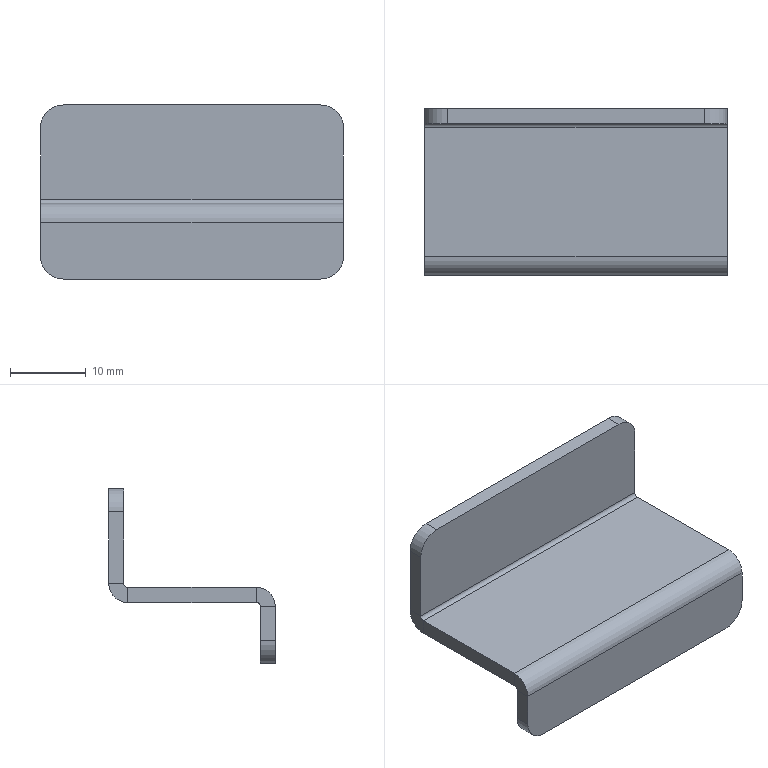Part | SolidWorks | features BaseBody 1 | 1 solid | 26 faces | box 40 x 22 x 23 mm | volume 3322 mm3 | plane 18 | cylinder 8 | commonest cylinder face diameters 6 x4 1 x2 5 x2
STEP:
#1=CARTESIAN_POINT('',(17.,-11.,-10.));
#2=VERTEX_POINT('',#1);
#3=CARTESIAN_POINT('',(20.,-11.,-7.));
#4=VERTEX_POINT('',#3);
#5=CARTESIAN_POINT('',(17.,-11.,-7.));
#6=DIRECTION('',(0.,-1.,0.));
#7=DIRECTION('',(0.,0.,-1.));
#8=AXIS2_PLACEMENT_3D('',#5,#6,#7);
#9=CIRCLE('',#8,3.);
#10=EDGE_CURVE('',#2,#4,#9,.T.);
#11=ORIENTED_EDGE('',*,*,#10,.F.);
#12=CARTESIAN_POINT('',(17.,-9.,-10.));
#13=VERTEX_POINT('',#12);
#14=CARTESIAN_POINT('',(17.,-11.,-10.));
#15=DIRECTION('',(0.,-1.,0.));
#16=VECTOR('',#15,1000.);
#17=LINE('',#14,#16);
#18=EDGE_CURVE('',#13,#2,#17,.T.);
#19=ORIENTED_EDGE('',*,*,#18,.F.);
#20=CARTESIAN_POINT('',(20.,-9.,-7.));
#21=VERTEX_POINT('',#20);
#22=CARTESIAN_POINT('',(17.,-9.,-7.));
#23=DIRECTION('',(0.,1.,0.));
#24=DIRECTION('',(0.,0.,-1.));
#25=AXIS2_PLACEMENT_3D('',#22,#23,#24);
#26=CIRCLE('',#25,3.);
#27=EDGE_CURVE('',#21,#13,#26,.T.);
#28=ORIENTED_EDGE('',*,*,#27,.F.);
#29=CARTESIAN_POINT('',(20.,-11.,-7.));
#30=DIRECTION('',(0.,1.,0.));
#31=VECTOR('',#30,1000.);
#32=LINE('',#29,#31);
#33=EDGE_CURVE('',#4,#21,#32,.T.);
#34=ORIENTED_EDGE('',*,*,#33,.F.);
#35=EDGE_LOOP('',(#11,#19,#28,#34));
#36=FACE_OUTER_BOUND('',#35,.T.);
#37=CARTESIAN_POINT('',(17.,-11.,-7.));
#38=DIRECTION('',(0.,1.,0.));
#39=DIRECTION('',(0.,0.,1.));
#40=AXIS2_PLACEMENT_3D('',#37,#38,#39);
#41=CYLINDRICAL_SURFACE('',#40,3.);
#42=ADVANCED_FACE('',(#36),#41,.T.);
#43=CARTESIAN_POINT('',(-20.,-11.,-7.));
#44=VERTEX_POINT('',#43);
#45=CARTESIAN_POINT('',(-17.,-11.,-10.));
#46=VERTEX_POINT('',#45);
#47=CARTESIAN_POINT('',(-17.,-11.,-7.));
#48=DIRECTION('',(0.,-1.,0.));
#49=DIRECTION('',(0.,0.,-1.));
#50=AXIS2_PLACEMENT_3D('',#47,#48,#49);
#51=CIRCLE('',#50,3.);
#52=EDGE_CURVE('',#44,#46,#51,.T.);
#53=ORIENTED_EDGE('',*,*,#52,.F.);
#54=CARTESIAN_POINT('',(-20.,-9.,-7.));
#55=VERTEX_POINT('',#54);
#56=CARTESIAN_POINT('',(-20.,-11.,-7.));
#57=DIRECTION('',(0.,-1.,0.));
#58=VECTOR('',#57,1000.);
#59=LINE('',#56,#58);
#60=EDGE_CURVE('',#55,#44,#59,.T.);
#61=ORIENTED_EDGE('',*,*,#60,.F.);
#62=CARTESIAN_POINT('',(-17.,-9.,-10.));
#63=VERTEX_POINT('',#62);
#64=CARTESIAN_POINT('',(-17.,-9.,-7.));
#65=DIRECTION('',(0.,1.,0.));
#66=DIRECTION('',(0.,0.,-1.));
#67=AXIS2_PLACEMENT_3D('',#64,#65,#66);
#68=CIRCLE('',#67,3.);
#69=EDGE_CURVE('',#63,#55,#68,.T.);
#70=ORIENTED_EDGE('',*,*,#69,.F.);
#71=CARTESIAN_POINT('',(-17.,-11.,-10.));
#72=DIRECTION('',(0.,1.,0.));
#73=VECTOR('',#72,1000.);
#74=LINE('',#71,#73);
#75=EDGE_CURVE('',#46,#63,#74,.T.);
#76=ORIENTED_EDGE('',*,*,#75,.F.);
#77=EDGE_LOOP('',(#53,#61,#70,#76));
#78=FACE_OUTER_BOUND('',#77,.T.);
#79=CARTESIAN_POINT('',(-17.,-11.,-7.));
#80=DIRECTION('',(0.,1.,0.));
#81=DIRECTION('',(0.,0.,1.));
#82=AXIS2_PLACEMENT_3D('',#79,#80,#81);
#83=CYLINDRICAL_SURFACE('',#82,3.);
#84=ADVANCED_FACE('',(#78),#83,.T.);
#85=CARTESIAN_POINT('',(17.,11.,13.));
#86=VERTEX_POINT('',#85);
#87=CARTESIAN_POINT('',(20.,11.,10.));
#88=VERTEX_POINT('',#87);
#89=CARTESIAN_POINT('',(17.,11.,10.));
#90=DIRECTION('',(0.,1.,0.));
#91=DIRECTION('',(0.,0.,-1.));
#92=AXIS2_PLACEMENT_3D('',#89,#90,#91);
#93=CIRCLE('',#92,3.);
#94=EDGE_CURVE('',#86,#88,#93,.T.);
#95=ORIENTED_EDGE('',*,*,#94,.F.);
#96=CARTESIAN_POINT('',(17.,9.,13.));
#97=VERTEX_POINT('',#96);
#98=CARTESIAN_POINT('',(17.,11.,13.));
#99=DIRECTION('',(0.,1.,0.));
#100=VECTOR('',#99,1000.);
#101=LINE('',#98,#100);
#102=EDGE_CURVE('',#97,#86,#101,.T.);
#103=ORIENTED_EDGE('',*,*,#102,.F.);
#104=CARTESIAN_POINT('',(20.,9.,10.));
#105=VERTEX_POINT('',#104);
#106=CARTESIAN_POINT('',(17.,9.,10.));
#107=DIRECTION('',(0.,-1.,0.));
#108=DIRECTION('',(0.,0.,-1.));
#109=AXIS2_PLACEMENT_3D('',#106,#107,#108);
#110=CIRCLE('',#109,3.);
#111=EDGE_CURVE('',#105,#97,#110,.T.);
#112=ORIENTED_EDGE('',*,*,#111,.F.);
#113=CARTESIAN_POINT('',(20.,11.,10.));
#114=DIRECTION('',(0.,-1.,0.));
#115=VECTOR('',#114,1000.);
#116=LINE('',#113,#115);
#117=EDGE_CURVE('',#88,#105,#116,.T.);
#118=ORIENTED_EDGE('',*,*,#117,.F.);
#119=EDGE_LOOP('',(#95,#103,#112,#118));
#120=FACE_OUTER_BOUND('',#119,.T.);
#121=CARTESIAN_POINT('',(17.,11.,10.));
#122=DIRECTION('',(0.,-1.,0.));
#123=DIRECTION('',(0.,0.,-1.));
#124=AXIS2_PLACEMENT_3D('',#121,#122,#123);
#125=CYLINDRICAL_SURFACE('',#124,3.);
#126=ADVANCED_FACE('',(#120),#125,.T.);
#127=CARTESIAN_POINT('',(-20.,11.,10.));
#128=VERTEX_POINT('',#127);
#129=CARTESIAN_POINT('',(-17.,11.,13.));
#130=VERTEX_POINT('',#129);
#131=CARTESIAN_POINT('',(-17.,11.,10.));
#132=DIRECTION('',(0.,1.,0.));
#133=DIRECTION('',(0.,0.,-1.));
#134=AXIS2_PLACEMENT_3D('',#131,#132,#133);
#135=CIRCLE('',#134,3.);
#136=EDGE_CURVE('',#128,#130,#135,.T.);
#137=ORIENTED_EDGE('',*,*,#136,.F.);
#138=CARTESIAN_POINT('',(-20.,9.,10.));
#139=VERTEX_POINT('',#138);
#140=CARTESIAN_POINT('',(-20.,11.,10.));
#141=DIRECTION('',(0.,1.,0.));
#142=VECTOR('',#141,1000.);
#143=LINE('',#140,#142);
#144=EDGE_CURVE('',#139,#128,#143,.T.);
#145=ORIENTED_EDGE('',*,*,#144,.F.);
#146=CARTESIAN_POINT('',(-17.,9.,13.));
#147=VERTEX_POINT('',#146);
#148=CARTESIAN_POINT('',(-17.,9.,10.));
#149=DIRECTION('',(0.,-1.,0.));
#150=DIRECTION('',(0.,0.,-1.));
#151=AXIS2_PLACEMENT_3D('',#148,#149,#150);
#152=CIRCLE('',#151,3.);
#153=EDGE_CURVE('',#147,#139,#152,.T.);
#154=ORIENTED_EDGE('',*,*,#153,.F.);
#155=CARTESIAN_POINT('',(-17.,11.,13.));
#156=DIRECTION('',(0.,-1.,0.));
#157=VECTOR('',#156,1000.);
#158=LINE('',#155,#157);
#159=EDGE_CURVE('',#130,#147,#158,.T.);
#160=ORIENTED_EDGE('',*,*,#159,.F.);
#161=EDGE_LOOP('',(#137,#145,#154,#160));
#162=FACE_OUTER_BOUND('',#161,.T.);
#163=CARTESIAN_POINT('',(-17.,11.,10.));
#164=DIRECTION('',(0.,-1.,0.));
#165=DIRECTION('',(0.,0.,-1.));
#166=AXIS2_PLACEMENT_3D('',#163,#164,#165);
#167=CYLINDRICAL_SURFACE('',#166,3.);
#168=ADVANCED_FACE('',(#162),#167,.T.);
#169=CARTESIAN_POINT('',(0.,11.,13.));
#170=DIRECTION('',(1.,0.,0.));
#171=VECTOR('',#170,1000.);
#172=LINE('',#169,#171);
#173=EDGE_CURVE('',#130,#86,#172,.T.);
#174=ORIENTED_EDGE('',*,*,#173,.F.);
#175=ORIENTED_EDGE('',*,*,#159,.T.);
#176=CARTESIAN_POINT('',(20.,9.,13.));
#177=DIRECTION('',(1.,0.,0.));
#178=VECTOR('',#177,1000.);
#179=LINE('',#176,#178);
#180=EDGE_CURVE('',#147,#97,#179,.T.);
#181=ORIENTED_EDGE('',*,*,#180,.T.);
#182=ORIENTED_EDGE('',*,*,#102,.T.);
#183=EDGE_LOOP('',(#174,#175,#181,#182));
#184=FACE_OUTER_BOUND('',#183,.T.);
#185=CARTESIAN_POINT('',(20.,11.,13.));
#186=DIRECTION('',(0.,0.,-1.));
#187=DIRECTION('',(0.,-1.,0.));
#188=AXIS2_PLACEMENT_3D('',#185,#186,#187);
#189=PLANE('',#188);
#190=ADVANCED_FACE('',(#184),#189,.F.);
#191=ORIENTED_EDGE('',*,*,#180,.F.);
#192=ORIENTED_EDGE('',*,*,#153,.T.);
#193=CARTESIAN_POINT('',(-20.,9.,0.5));
#194=VERTEX_POINT('',#193);
#195=CARTESIAN_POINT('',(-20.,9.,13.));
#196=DIRECTION('',(0.,0.,1.));
#197=VECTOR('',#196,1000.);
#198=LINE('',#195,#197);
#199=EDGE_CURVE('',#194,#139,#198,.T.);
#200=ORIENTED_EDGE('',*,*,#199,.F.);
#201=CARTESIAN_POINT('',(20.,9.,0.5));
#202=VERTEX_POINT('',#201);
#203=CARTESIAN_POINT('',(20.,9.,0.5));
#204=DIRECTION('',(-1.,0.,0.));
#205=VECTOR('',#204,1000.);
#206=LINE('',#203,#205);
#207=EDGE_CURVE('',#202,#194,#206,.T.);
#208=ORIENTED_EDGE('',*,*,#207,.F.);
#209=CARTESIAN_POINT('',(20.,9.,0.));
#210=DIRECTION('',(0.,0.,-1.));
#211=VECTOR('',#210,1000.);
#212=LINE('',#209,#211);
#213=EDGE_CURVE('',#105,#202,#212,.T.);
#214=ORIENTED_EDGE('',*,*,#213,.F.);
#215=ORIENTED_EDGE('',*,*,#111,.T.);
#216=EDGE_LOOP('',(#191,#192,#200,#208,#214,#215));
#217=FACE_OUTER_BOUND('',#216,.T.);
#218=CARTESIAN_POINT('',(0.,9.,0.));
#219=DIRECTION('',(0.,-1.,0.));
#220=DIRECTION('',(-1.,0.,0.));
#221=AXIS2_PLACEMENT_3D('',#218,#219,#220);
#222=PLANE('',#221);
#223=ADVANCED_FACE('',(#217),#222,.T.);
#224=CARTESIAN_POINT('',(-20.,11.,0.5));
#225=VERTEX_POINT('',#224);
#226=CARTESIAN_POINT('',(-20.,11.,0.));
#227=DIRECTION('',(0.,0.,1.));
#228=VECTOR('',#227,1000.);
#229=LINE('',#226,#228);
#230=EDGE_CURVE('',#225,#128,#229,.T.);
#231=ORIENTED_EDGE('',*,*,#230,.T.);
#232=ORIENTED_EDGE('',*,*,#136,.T.);
#233=ORIENTED_EDGE('',*,*,#173,.T.);
#234=ORIENTED_EDGE('',*,*,#94,.T.);
#235=CARTESIAN_POINT('',(20.,11.,0.5));
#236=VERTEX_POINT('',#235);
#237=CARTESIAN_POINT('',(20.,11.,0.));
#238=DIRECTION('',(0.,0.,-1.));
#239=VECTOR('',#238,1000.);
#240=LINE('',#237,#239);
#241=EDGE_CURVE('',#88,#236,#240,.T.);
#242=ORIENTED_EDGE('',*,*,#241,.T.);
#243=CARTESIAN_POINT('',(20.,11.,0.5));
#244=DIRECTION('',(1.,0.,0.));
#245=VECTOR('',#244,1000.);
#246=LINE('',#243,#245);
#247=EDGE_CURVE('',#225,#236,#246,.T.);
#248=ORIENTED_EDGE('',*,*,#247,.F.);
#249=EDGE_LOOP('',(#231,#232,#233,#234,#242,#248));
#250=FACE_OUTER_BOUND('',#249,.T.);
#251=CARTESIAN_POINT('',(0.,11.,0.));
#252=DIRECTION('',(0.,-1.,0.));
#253=DIRECTION('',(-1.,0.,0.));
#254=AXIS2_PLACEMENT_3D('',#251,#252,#253);
#255=PLANE('',#254);
#256=ADVANCED_FACE('',(#250),#255,.F.);
#257=ORIENTED_EDGE('',*,*,#199,.T.);
#258=ORIENTED_EDGE('',*,*,#144,.T.);
#259=ORIENTED_EDGE('',*,*,#230,.F.);
#260=CARTESIAN_POINT('',(-20.,9.,0.5));
#261=DIRECTION('',(0.,1.,0.));
#262=VECTOR('',#261,1000.);
#263=LINE('',#260,#262);
#264=EDGE_CURVE('',#194,#225,#263,.T.);
#265=ORIENTED_EDGE('',*,*,#264,.F.);
#266=EDGE_LOOP('',(#257,#258,#259,#265));
#267=FACE_OUTER_BOUND('',#266,.T.);
#268=CARTESIAN_POINT('',(-20.,11.,13.));
#269=DIRECTION('',(1.,0.,0.));
#270=DIRECTION('',(0.,1.,0.));
#271=AXIS2_PLACEMENT_3D('',#268,#269,#270);
#272=PLANE('',#271);
#273=ADVANCED_FACE('',(#267),#272,.F.);
#274=ORIENTED_EDGE('',*,*,#241,.F.);
#275=ORIENTED_EDGE('',*,*,#117,.T.);
#276=ORIENTED_EDGE('',*,*,#213,.T.);
#277=CARTESIAN_POINT('',(20.,11.,0.5));
#278=DIRECTION('',(0.,1.,0.));
#279=VECTOR('',#278,1000.);
#280=LINE('',#277,#279);
#281=EDGE_CURVE('',#202,#236,#280,.T.);
#282=ORIENTED_EDGE('',*,*,#281,.T.);
#283=EDGE_LOOP('',(#274,#275,#276,#282));
#284=FACE_OUTER_BOUND('',#283,.T.);
#285=CARTESIAN_POINT('',(20.,11.,0.));
#286=DIRECTION('',(-1.,0.,0.));
#287=DIRECTION('',(0.,0.,1.));
#288=AXIS2_PLACEMENT_3D('',#285,#286,#287);
#289=PLANE('',#288);
#290=ADVANCED_FACE('',(#284),#289,.F.);
#291=CARTESIAN_POINT('',(-20.,8.5,0.));
#292=VERTEX_POINT('',#291);
#293=CARTESIAN_POINT('',(20.,8.5,0.));
#294=VERTEX_POINT('',#293);
#295=CARTESIAN_POINT('',(-20.,8.5,0.));
#296=DIRECTION('',(1.,0.,0.));
#297=VECTOR('',#296,1000.);
#298=LINE('',#295,#297);
#299=EDGE_CURVE('',#292,#294,#298,.T.);
#300=ORIENTED_EDGE('',*,*,#299,.T.);
#301=CARTESIAN_POINT('',(20.,8.5,0.5));
#302=DIRECTION('',(1.,0.,0.));
#303=DIRECTION('',(0.,0.,1.));
#304=AXIS2_PLACEMENT_3D('',#301,#302,#303);
#305=CIRCLE('',#304,0.5);
#306=EDGE_CURVE('',#294,#202,#305,.T.);
#307=ORIENTED_EDGE('',*,*,#306,.T.);
#308=ORIENTED_EDGE('',*,*,#207,.T.);
#309=CARTESIAN_POINT('',(-20.,8.5,0.5));
#310=DIRECTION('',(-1.,0.,0.));
#311=DIRECTION('',(0.,0.,1.));
#312=AXIS2_PLACEMENT_3D('',#309,#310,#311);
#313=CIRCLE('',#312,0.5);
#314=EDGE_CURVE('',#194,#292,#313,.T.);
#315=ORIENTED_EDGE('',*,*,#314,.T.);
#316=EDGE_LOOP('',(#300,#307,#308,#315));
#317=FACE_OUTER_BOUND('',#316,.T.);
#318=CARTESIAN_POINT('',(-20.,8.5,0.5));
#319=DIRECTION('',(-1.,0.,0.));
#320=DIRECTION('',(0.,1.,0.));
#321=AXIS2_PLACEMENT_3D('',#318,#319,#320);
#322=CYLINDRICAL_SURFACE('',#321,0.5);
#323=ADVANCED_FACE('',(#317),#322,.F.);
#324=CARTESIAN_POINT('',(-20.,8.5,-2.));
#325=VERTEX_POINT('',#324);
#326=CARTESIAN_POINT('',(20.,8.5,-2.));
#327=VERTEX_POINT('',#326);
#328=CARTESIAN_POINT('',(-20.,8.5,-2.));
#329=DIRECTION('',(1.,0.,0.));
#330=VECTOR('',#329,1000.);
#331=LINE('',#328,#330);
#332=EDGE_CURVE('',#325,#327,#331,.T.);
#333=ORIENTED_EDGE('',*,*,#332,.F.);
#334=CARTESIAN_POINT('',(-20.,8.5,0.5));
#335=DIRECTION('',(-1.,0.,0.));
#336=DIRECTION('',(0.,0.,1.));
#337=AXIS2_PLACEMENT_3D('',#334,#335,#336);
#338=CIRCLE('',#337,2.5);
#339=EDGE_CURVE('',#225,#325,#338,.T.);
#340=ORIENTED_EDGE('',*,*,#339,.F.);
#341=ORIENTED_EDGE('',*,*,#247,.T.);
#342=CARTESIAN_POINT('',(20.,8.5,0.5));
#343=DIRECTION('',(1.,0.,0.));
#344=DIRECTION('',(0.,0.,1.));
#345=AXIS2_PLACEMENT_3D('',#342,#343,#344);
#346=CIRCLE('',#345,2.5);
#347=EDGE_CURVE('',#327,#236,#346,.T.);
#348=ORIENTED_EDGE('',*,*,#347,.F.);
#349=EDGE_LOOP('',(#333,#340,#341,#348));
#350=FACE_OUTER_BOUND('',#349,.T.);
#351=CARTESIAN_POINT('',(-20.,8.5,0.5));
#352=DIRECTION('',(-1.,0.,0.));
#353=DIRECTION('',(0.,1.,0.));
#354=AXIS2_PLACEMENT_3D('',#351,#352,#353);
#355=CYLINDRICAL_SURFACE('',#354,2.5);
#356=ADVANCED_FACE('',(#350),#355,.T.);
#357=ORIENTED_EDGE('',*,*,#314,.F.);
#358=ORIENTED_EDGE('',*,*,#264,.T.);
#359=ORIENTED_EDGE('',*,*,#339,.T.);
#360=CARTESIAN_POINT('',(-20.,8.5,0.));
#361=DIRECTION('',(0.,0.,-1.));
#362=VECTOR('',#361,1000.);
#363=LINE('',#360,#362);
#364=EDGE_CURVE('',#292,#325,#363,.T.);
#365=ORIENTED_EDGE('',*,*,#364,.F.);
#366=EDGE_LOOP('',(#357,#358,#359,#365));
#367=FACE_OUTER_BOUND('',#366,.T.);
#368=CARTESIAN_POINT('',(-20.,8.5,0.5));
#369=DIRECTION('',(1.,0.,0.));
#370=DIRECTION('',(0.,1.,0.));
#371=AXIS2_PLACEMENT_3D('',#368,#369,#370);
#372=PLANE('',#371);
#373=ADVANCED_FACE('',(#367),#372,.F.);
#374=ORIENTED_EDGE('',*,*,#281,.F.);
#375=ORIENTED_EDGE('',*,*,#306,.F.);
#376=CARTESIAN_POINT('',(20.,8.5,0.));
#377=DIRECTION('',(0.,0.,-1.));
#378=VECTOR('',#377,1000.);
#379=LINE('',#376,#378);
#380=EDGE_CURVE('',#294,#327,#379,.T.);
#381=ORIENTED_EDGE('',*,*,#380,.T.);
#382=ORIENTED_EDGE('',*,*,#347,.T.);
#383=EDGE_LOOP('',(#374,#375,#381,#382));
#384=FACE_OUTER_BOUND('',#383,.T.);
#385=CARTESIAN_POINT('',(20.,8.5,0.5));
#386=DIRECTION('',(1.,0.,0.));
#387=DIRECTION('',(0.,1.,0.));
#388=AXIS2_PLACEMENT_3D('',#385,#386,#387);
#389=PLANE('',#388);
#390=ADVANCED_FACE('',(#384),#389,.T.);
#391=CARTESIAN_POINT('',(-20.,-11.,-10.));
#392=DIRECTION('',(-1.,0.,0.));
#393=VECTOR('',#392,1000.);
#394=LINE('',#391,#393);
#395=EDGE_CURVE('',#2,#46,#394,.T.);
#396=ORIENTED_EDGE('',*,*,#395,.T.);
#397=ORIENTED_EDGE('',*,*,#75,.T.);
#398=CARTESIAN_POINT('',(0.,-9.,-10.));
#399=DIRECTION('',(-1.,0.,0.));
#400=VECTOR('',#399,1000.);
#401=LINE('',#398,#400);
#402=EDGE_CURVE('',#13,#63,#401,.T.);
#403=ORIENTED_EDGE('',*,*,#402,.F.);
#404=ORIENTED_EDGE('',*,*,#18,.T.);
#405=EDGE_LOOP('',(#396,#397,#403,#404));
#406=FACE_OUTER_BOUND('',#405,.T.);
#407=CARTESIAN_POINT('',(-20.,-11.,-10.));
#408=DIRECTION('',(0.,0.,-1.));
#409=DIRECTION('',(0.,-1.,0.));
#410=AXIS2_PLACEMENT_3D('',#407,#408,#409);
#411=PLANE('',#410);
#412=ADVANCED_FACE('',(#406),#411,.T.);
#413=ORIENTED_EDGE('',*,*,#402,.T.);
#414=ORIENTED_EDGE('',*,*,#69,.T.);
#415=CARTESIAN_POINT('',(-20.,-9.,-2.5));
#416=VERTEX_POINT('',#415);
#417=CARTESIAN_POINT('',(-20.,-9.,0.));
#418=DIRECTION('',(0.,0.,1.));
#419=VECTOR('',#418,1000.);
#420=LINE('',#417,#419);
#421=EDGE_CURVE('',#55,#416,#420,.T.);
#422=ORIENTED_EDGE('',*,*,#421,.T.);
#423=CARTESIAN_POINT('',(20.,-9.,-2.5));
#424=VERTEX_POINT('',#423);
#425=CARTESIAN_POINT('',(20.,-9.,-2.5));
#426=DIRECTION('',(-1.,0.,0.));
#427=VECTOR('',#426,1000.);
#428=LINE('',#425,#427);
#429=EDGE_CURVE('',#424,#416,#428,.T.);
#430=ORIENTED_EDGE('',*,*,#429,.F.);
#431=CARTESIAN_POINT('',(20.,-9.,0.));
#432=DIRECTION('',(0.,0.,-1.));
#433=VECTOR('',#432,1000.);
#434=LINE('',#431,#433);
#435=EDGE_CURVE('',#424,#21,#434,.T.);
#436=ORIENTED_EDGE('',*,*,#435,.T.);
#437=ORIENTED_EDGE('',*,*,#27,.T.);
#438=EDGE_LOOP('',(#413,#414,#422,#430,#436,#437));
#439=FACE_OUTER_BOUND('',#438,.T.);
#440=CARTESIAN_POINT('',(0.,-9.,0.));
#441=DIRECTION('',(0.,-1.,0.));
#442=DIRECTION('',(-1.,0.,0.));
#443=AXIS2_PLACEMENT_3D('',#440,#441,#442);
#444=PLANE('',#443);
#445=ADVANCED_FACE('',(#439),#444,.F.);
#446=CARTESIAN_POINT('',(-20.,-11.,-2.5));
#447=VERTEX_POINT('',#446);
#448=CARTESIAN_POINT('',(-20.,-11.,-2.));
#449=DIRECTION('',(0.,0.,1.));
#450=VECTOR('',#449,1000.);
#451=LINE('',#448,#450);
#452=EDGE_CURVE('',#44,#447,#451,.T.);
#453=ORIENTED_EDGE('',*,*,#452,.F.);
#454=ORIENTED_EDGE('',*,*,#52,.T.);
#455=ORIENTED_EDGE('',*,*,#395,.F.);
#456=ORIENTED_EDGE('',*,*,#10,.T.);
#457=CARTESIAN_POINT('',(20.,-11.,-2.5));
#458=VERTEX_POINT('',#457);
#459=CARTESIAN_POINT('',(20.,-11.,-10.));
#460=DIRECTION('',(0.,0.,-1.));
#461=VECTOR('',#460,1000.);
#462=LINE('',#459,#461);
#463=EDGE_CURVE('',#458,#4,#462,.T.);
#464=ORIENTED_EDGE('',*,*,#463,.F.);
#465=CARTESIAN_POINT('',(0.,-11.,-2.5));
#466=DIRECTION('',(-1.,0.,0.));
#467=VECTOR('',#466,1000.);
#468=LINE('',#465,#467);
#469=EDGE_CURVE('',#458,#447,#468,.T.);
#470=ORIENTED_EDGE('',*,*,#469,.T.);
#471=EDGE_LOOP('',(#453,#454,#455,#456,#464,#470));
#472=FACE_OUTER_BOUND('',#471,.T.);
#473=CARTESIAN_POINT('',(0.,-11.,0.));
#474=DIRECTION('',(0.,-1.,0.));
#475=DIRECTION('',(-1.,0.,0.));
#476=AXIS2_PLACEMENT_3D('',#473,#474,#475);
#477=PLANE('',#476);
#478=ADVANCED_FACE('',(#472),#477,.T.);
#479=ORIENTED_EDGE('',*,*,#463,.T.);
#480=ORIENTED_EDGE('',*,*,#33,.T.);
#481=ORIENTED_EDGE('',*,*,#435,.F.);
#482=CARTESIAN_POINT('',(20.,-11.,-2.5));
#483=DIRECTION('',(0.,-1.,0.));
#484=VECTOR('',#483,1000.);
#485=LINE('',#482,#484);
#486=EDGE_CURVE('',#424,#458,#485,.T.);
#487=ORIENTED_EDGE('',*,*,#486,.T.);
#488=EDGE_LOOP('',(#479,#480,#481,#487));
#489=FACE_OUTER_BOUND('',#488,.T.);
#490=CARTESIAN_POINT('',(20.,-11.,-10.));
#491=DIRECTION('',(1.,0.,0.));
#492=DIRECTION('',(0.,1.,0.));
#493=AXIS2_PLACEMENT_3D('',#490,#491,#492);
#494=PLANE('',#493);
#495=ADVANCED_FACE('',(#489),#494,.T.);
#496=ORIENTED_EDGE('',*,*,#421,.F.);
#497=ORIENTED_EDGE('',*,*,#60,.T.);
#498=ORIENTED_EDGE('',*,*,#452,.T.);
#499=CARTESIAN_POINT('',(-20.,-9.,-2.5));
#500=DIRECTION('',(0.,-1.,0.));
#501=VECTOR('',#500,1000.);
#502=LINE('',#499,#501);
#503=EDGE_CURVE('',#416,#447,#502,.T.);
#504=ORIENTED_EDGE('',*,*,#503,.F.);
#505=EDGE_LOOP('',(#496,#497,#498,#504));
#506=FACE_OUTER_BOUND('',#505,.T.);
#507=CARTESIAN_POINT('',(-20.,-11.,-2.));
#508=DIRECTION('',(-1.,0.,0.));
#509=DIRECTION('',(0.,0.,1.));
#510=AXIS2_PLACEMENT_3D('',#507,#508,#509);
#511=PLANE('',#510);
#512=ADVANCED_FACE('',(#506),#511,.T.);
#513=CARTESIAN_POINT('',(-20.,-8.5,-2.));
#514=VERTEX_POINT('',#513);
#515=CARTESIAN_POINT('',(20.,-8.5,-2.));
#516=VERTEX_POINT('',#515);
#517=CARTESIAN_POINT('',(-20.,-8.5,-2.));
#518=DIRECTION('',(1.,0.,0.));
#519=VECTOR('',#518,1000.);
#520=LINE('',#517,#519);
#521=EDGE_CURVE('',#514,#516,#520,.T.);
#522=ORIENTED_EDGE('',*,*,#521,.T.);
#523=CARTESIAN_POINT('',(20.,-8.5,-2.5));
#524=DIRECTION('',(1.,0.,0.));
#525=DIRECTION('',(0.,0.,1.));
#526=AXIS2_PLACEMENT_3D('',#523,#524,#525);
#527=CIRCLE('',#526,0.5);
#528=EDGE_CURVE('',#516,#424,#527,.T.);
#529=ORIENTED_EDGE('',*,*,#528,.T.);
#530=ORIENTED_EDGE('',*,*,#429,.T.);
#531=CARTESIAN_POINT('',(-20.,-8.5,-2.5));
#532=DIRECTION('',(-1.,0.,0.));
#533=DIRECTION('',(0.,0.,1.));
#534=AXIS2_PLACEMENT_3D('',#531,#532,#533);
#535=CIRCLE('',#534,0.5);
#536=EDGE_CURVE('',#416,#514,#535,.T.);
#537=ORIENTED_EDGE('',*,*,#536,.T.);
#538=EDGE_LOOP('',(#522,#529,#530,#537));
#539=FACE_OUTER_BOUND('',#538,.T.);
#540=CARTESIAN_POINT('',(-20.,-8.5,-2.5));
#541=DIRECTION('',(-1.,0.,0.));
#542=DIRECTION('',(0.,-1.,0.));
#543=AXIS2_PLACEMENT_3D('',#540,#541,#542);
#544=CYLINDRICAL_SURFACE('',#543,0.5);
#545=ADVANCED_FACE('',(#539),#544,.F.);
#546=CARTESIAN_POINT('',(-20.,-8.5,0.));
#547=VERTEX_POINT('',#546);
#548=CARTESIAN_POINT('',(20.,-8.5,0.));
#549=VERTEX_POINT('',#548);
#550=CARTESIAN_POINT('',(-20.,-8.5,0.));
#551=DIRECTION('',(1.,0.,0.));
#552=VECTOR('',#551,1000.);
#553=LINE('',#550,#552);
#554=EDGE_CURVE('',#547,#549,#553,.T.);
#555=ORIENTED_EDGE('',*,*,#554,.F.);
#556=CARTESIAN_POINT('',(-20.,-8.5,-2.5));
#557=DIRECTION('',(-1.,0.,0.));
#558=DIRECTION('',(0.,0.,1.));
#559=AXIS2_PLACEMENT_3D('',#556,#557,#558);
#560=CIRCLE('',#559,2.5);
#561=EDGE_CURVE('',#447,#547,#560,.T.);
#562=ORIENTED_EDGE('',*,*,#561,.F.);
#563=ORIENTED_EDGE('',*,*,#469,.F.);
#564=CARTESIAN_POINT('',(20.,-8.5,-2.5));
#565=DIRECTION('',(1.,0.,0.));
#566=DIRECTION('',(0.,0.,1.));
#567=AXIS2_PLACEMENT_3D('',#564,#565,#566);
#568=CIRCLE('',#567,2.5);
#569=EDGE_CURVE('',#549,#458,#568,.T.);
#570=ORIENTED_EDGE('',*,*,#569,.F.);
#571=EDGE_LOOP('',(#555,#562,#563,#570));
#572=FACE_OUTER_BOUND('',#571,.T.);
#573=CARTESIAN_POINT('',(-20.,-8.5,-2.5));
#574=DIRECTION('',(-1.,0.,0.));
#575=DIRECTION('',(0.,-1.,0.));
#576=AXIS2_PLACEMENT_3D('',#573,#574,#575);
#577=CYLINDRICAL_SURFACE('',#576,2.5);
#578=ADVANCED_FACE('',(#572),#577,.T.);
#579=ORIENTED_EDGE('',*,*,#536,.F.);
#580=ORIENTED_EDGE('',*,*,#503,.T.);
#581=ORIENTED_EDGE('',*,*,#561,.T.);
#582=CARTESIAN_POINT('',(-20.,-8.5,-2.));
#583=DIRECTION('',(0.,0.,1.));
#584=VECTOR('',#583,1000.);
#585=LINE('',#582,#584);
#586=EDGE_CURVE('',#514,#547,#585,.T.);
#587=ORIENTED_EDGE('',*,*,#586,.F.);
#588=EDGE_LOOP('',(#579,#580,#581,#587));
#589=FACE_OUTER_BOUND('',#588,.T.);
#590=CARTESIAN_POINT('',(-20.,-8.5,-2.5));
#591=DIRECTION('',(1.,0.,0.));
#592=DIRECTION('',(0.,1.,0.));
#593=AXIS2_PLACEMENT_3D('',#590,#591,#592);
#594=PLANE('',#593);
#595=ADVANCED_FACE('',(#589),#594,.F.);
#596=ORIENTED_EDGE('',*,*,#486,.F.);
#597=ORIENTED_EDGE('',*,*,#528,.F.);
#598=CARTESIAN_POINT('',(20.,-8.5,-2.));
#599=DIRECTION('',(0.,0.,1.));
#600=VECTOR('',#599,1000.);
#601=LINE('',#598,#600);
#602=EDGE_CURVE('',#516,#549,#601,.T.);
#603=ORIENTED_EDGE('',*,*,#602,.T.);
#604=ORIENTED_EDGE('',*,*,#569,.T.);
#605=EDGE_LOOP('',(#596,#597,#603,#604));
#606=FACE_OUTER_BOUND('',#605,.T.);
#607=CARTESIAN_POINT('',(20.,-8.5,-2.5));
#608=DIRECTION('',(1.,0.,0.));
#609=DIRECTION('',(0.,1.,0.));
#610=AXIS2_PLACEMENT_3D('',#607,#608,#609);
#611=PLANE('',#610);
#612=ADVANCED_FACE('',(#606),#611,.T.);
#613=ORIENTED_EDGE('',*,*,#380,.F.);
#614=CARTESIAN_POINT('',(20.,11.,0.));
#615=DIRECTION('',(0.,1.,0.));
#616=VECTOR('',#615,1000.);
#617=LINE('',#614,#616);
#618=EDGE_CURVE('',#549,#294,#617,.T.);
#619=ORIENTED_EDGE('',*,*,#618,.F.);
#620=ORIENTED_EDGE('',*,*,#602,.F.);
#621=CARTESIAN_POINT('',(20.,11.,-2.));
#622=DIRECTION('',(0.,1.,0.));
#623=VECTOR('',#622,1000.);
#624=LINE('',#621,#623);
#625=EDGE_CURVE('',#516,#327,#624,.T.);
#626=ORIENTED_EDGE('',*,*,#625,.T.);
#627=EDGE_LOOP('',(#613,#619,#620,#626));
#628=FACE_OUTER_BOUND('',#627,.T.);
#629=CARTESIAN_POINT('',(20.,11.,-2.));
#630=DIRECTION('',(1.,0.,0.));
#631=DIRECTION('',(0.,1.,0.));
#632=AXIS2_PLACEMENT_3D('',#629,#630,#631);
#633=PLANE('',#632);
#634=ADVANCED_FACE('',(#628),#633,.T.);
#635=ORIENTED_EDGE('',*,*,#618,.T.);
#636=ORIENTED_EDGE('',*,*,#299,.F.);
#637=CARTESIAN_POINT('',(-20.,11.,0.));
#638=DIRECTION('',(0.,-1.,0.));
#639=VECTOR('',#638,1000.);
#640=LINE('',#637,#639);
#641=EDGE_CURVE('',#292,#547,#640,.T.);
#642=ORIENTED_EDGE('',*,*,#641,.T.);
#643=ORIENTED_EDGE('',*,*,#554,.T.);
#644=EDGE_LOOP('',(#635,#636,#642,#643));
#645=FACE_OUTER_BOUND('',#644,.T.);
#646=CARTESIAN_POINT('',(0.,0.,0.));
#647=DIRECTION('',(0.,0.,1.));
#648=DIRECTION('',(1.,0.,0.));
#649=AXIS2_PLACEMENT_3D('',#646,#647,#648);
#650=PLANE('',#649);
#651=ADVANCED_FACE('',(#645),#650,.T.);
#652=ORIENTED_EDGE('',*,*,#332,.T.);
#653=ORIENTED_EDGE('',*,*,#625,.F.);
#654=ORIENTED_EDGE('',*,*,#521,.F.);
#655=CARTESIAN_POINT('',(-20.,11.,-2.));
#656=DIRECTION('',(0.,-1.,0.));
#657=VECTOR('',#656,1000.);
#658=LINE('',#655,#657);
#659=EDGE_CURVE('',#325,#514,#658,.T.);
#660=ORIENTED_EDGE('',*,*,#659,.F.);
#661=EDGE_LOOP('',(#652,#653,#654,#660));
#662=FACE_OUTER_BOUND('',#661,.T.);
#663=CARTESIAN_POINT('',(0.,0.,-2.));
#664=DIRECTION('',(0.,0.,1.));
#665=DIRECTION('',(1.,0.,0.));
#666=AXIS2_PLACEMENT_3D('',#663,#664,#665);
#667=PLANE('',#666);
#668=ADVANCED_FACE('',(#662),#667,.F.);
#669=ORIENTED_EDGE('',*,*,#641,.F.);
#670=ORIENTED_EDGE('',*,*,#364,.T.);
#671=ORIENTED_EDGE('',*,*,#659,.T.);
#672=ORIENTED_EDGE('',*,*,#586,.T.);
#673=EDGE_LOOP('',(#669,#670,#671,#672));
#674=FACE_OUTER_BOUND('',#673,.T.);
#675=CARTESIAN_POINT('',(-20.,11.,-2.));
#676=DIRECTION('',(-1.,0.,0.));
#677=DIRECTION('',(0.,1.,0.));
#678=AXIS2_PLACEMENT_3D('',#675,#676,#677);
#679=PLANE('',#678);
#680=ADVANCED_FACE('',(#674),#679,.T.);
#681=CLOSED_SHELL('',(#42,#84,#126,#168,#190,#223,#256,#273,#290,#323,#356,#373,#390,#412,#445,#478,#495,#512,#545,#578,#595,#612,#634,#651,#668,#680));
#682=MANIFOLD_SOLID_BREP('',#681);
#683=CARTESIAN_POINT('',(0.,0.,0.));
#684=DIRECTION('',(0.,0.,1.));
#685=DIRECTION('',(1.,0.,0.));
#686=AXIS2_PLACEMENT_3D('',#683,#684,#685);
#687=(LENGTH_UNIT()NAMED_UNIT(*)SI_UNIT(.MILLI.,.METRE.));
#688=UNCERTAINTY_MEASURE_WITH_UNIT(LENGTH_MEASURE(0.00001),#687,'','');
#689=(NAMED_UNIT(*)PLANE_ANGLE_UNIT()SI_UNIT($,.RADIAN.));
#690=(NAMED_UNIT(*)SI_UNIT($,.STERADIAN.)SOLID_ANGLE_UNIT());
#691=(GEOMETRIC_REPRESENTATION_CONTEXT(3)GLOBAL_UNCERTAINTY_ASSIGNED_CONTEXT((#688))GLOBAL_UNIT_ASSIGNED_CONTEXT((#687,#689,#690))REPRESENTATION_CONTEXT('',''));
#692=ADVANCED_BREP_SHAPE_REPRESENTATION('',(#682,#686),#691);